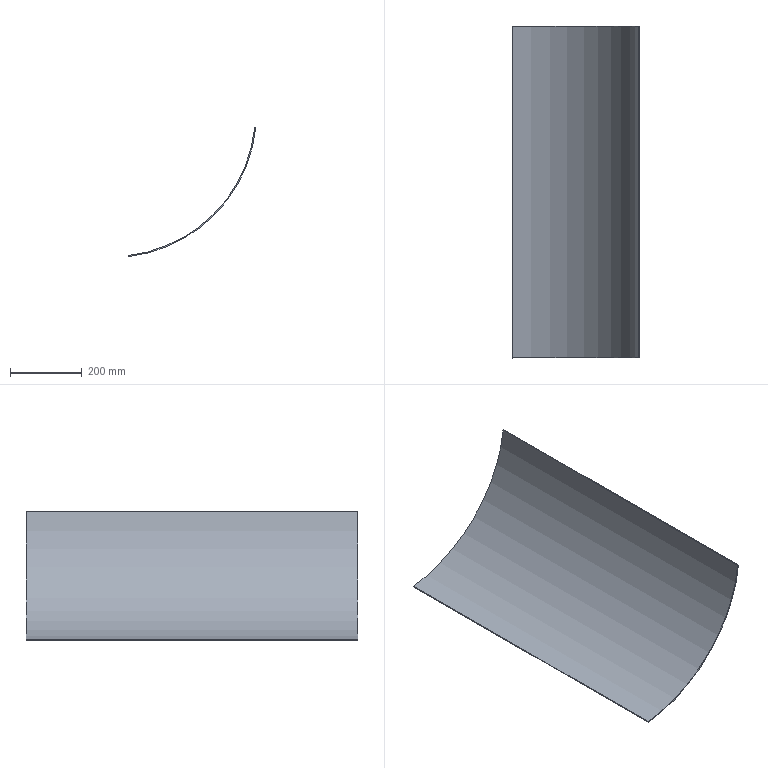Part | NX | features DATUM_CSYS 2, EXTRUDE 1, SKETCH 1 | 1 solid | 6 faces | box 355.98 x 926 x 360.442 mm | volume 1514546 mm3 | plane 4 | cylinder 2 | commonest cylinder face diameters 800 x1 806 x1
STEP:
#1=CARTESIAN_POINT('',(45.,463.,-397.461));
#2=VERTEX_POINT('',#1);
#3=CARTESIAN_POINT('',(45.337,463.,-400.442));
#4=VERTEX_POINT('',#3);
#5=CARTESIAN_POINT('',(45.,463.,-397.461));
#6=DIRECTION('',(0.1125,0.,-0.9937));
#7=VECTOR('',#6,1000.);
#8=LINE('',#5,#7);
#9=EDGE_CURVE('',#2,#4,#8,.T.);
#10=ORIENTED_EDGE('',*,*,#9,.F.);
#11=CARTESIAN_POINT('',(397.995,463.,-40.));
#12=VERTEX_POINT('',#11);
#13=CARTESIAN_POINT('',(0.,463.,0.));
#14=DIRECTION('',(0.,-1.,0.));
#15=DIRECTION('',(1.,0.,0.));
#16=AXIS2_PLACEMENT_3D('',#13,#14,#15);
#17=CIRCLE('',#16,400.);
#18=EDGE_CURVE('',#2,#12,#17,.T.);
#19=ORIENTED_EDGE('',*,*,#18,.T.);
#20=CARTESIAN_POINT('',(400.98,463.,-40.3));
#21=VERTEX_POINT('',#20);
#22=CARTESIAN_POINT('',(397.995,463.,-40.));
#23=DIRECTION('',(0.995,0.,-0.1));
#24=VECTOR('',#23,1000.);
#25=LINE('',#22,#24);
#26=EDGE_CURVE('',#12,#21,#25,.T.);
#27=ORIENTED_EDGE('',*,*,#26,.T.);
#28=CARTESIAN_POINT('',(0.,463.,0.));
#29=DIRECTION('',(0.,-1.,0.));
#30=DIRECTION('',(0.,0.,-1.));
#31=AXIS2_PLACEMENT_3D('',#28,#29,#30);
#32=CIRCLE('',#31,403.);
#33=EDGE_CURVE('',#4,#21,#32,.T.);
#34=ORIENTED_EDGE('',*,*,#33,.F.);
#35=EDGE_LOOP('',(#10,#19,#27,#34));
#36=FACE_BOUND('',#35,.T.);
#37=CARTESIAN_POINT('',(0.,463.,0.));
#38=DIRECTION('',(0.,1.,0.));
#39=DIRECTION('',(0.,0.,1.));
#40=AXIS2_PLACEMENT_3D('',#37,#38,#39);
#41=PLANE('',#40);
#42=ADVANCED_FACE('',(#36),#41,.T.);
#43=ORIENTED_EDGE('',*,*,#26,.F.);
#44=CARTESIAN_POINT('',(397.995,-463.,-40.));
#45=VERTEX_POINT('',#44);
#46=CARTESIAN_POINT('',(397.995,463.,-40.));
#47=DIRECTION('',(0.,-1.,0.));
#48=VECTOR('',#47,1000.);
#49=LINE('',#46,#48);
#50=EDGE_CURVE('',#12,#45,#49,.T.);
#51=ORIENTED_EDGE('',*,*,#50,.T.);
#52=CARTESIAN_POINT('',(400.98,-463.,-40.3));
#53=VERTEX_POINT('',#52);
#54=CARTESIAN_POINT('',(397.995,-463.,-40.));
#55=DIRECTION('',(0.995,0.,-0.1));
#56=VECTOR('',#55,1000.);
#57=LINE('',#54,#56);
#58=EDGE_CURVE('',#45,#53,#57,.T.);
#59=ORIENTED_EDGE('',*,*,#58,.T.);
#60=CARTESIAN_POINT('',(400.98,463.,-40.3));
#61=DIRECTION('',(0.,-1.,0.));
#62=VECTOR('',#61,1000.);
#63=LINE('',#60,#62);
#64=EDGE_CURVE('',#21,#53,#63,.T.);
#65=ORIENTED_EDGE('',*,*,#64,.F.);
#66=EDGE_LOOP('',(#43,#51,#59,#65));
#67=FACE_BOUND('',#66,.T.);
#68=CARTESIAN_POINT('',(397.995,0.,-40.));
#69=DIRECTION('',(0.1,0.,0.995));
#70=DIRECTION('',(0.,-1.,0.));
#71=AXIS2_PLACEMENT_3D('',#68,#69,#70);
#72=PLANE('',#71);
#73=ADVANCED_FACE('',(#67),#72,.T.);
#74=ORIENTED_EDGE('',*,*,#58,.F.);
#75=CARTESIAN_POINT('',(45.,-463.,-397.461));
#76=VERTEX_POINT('',#75);
#77=CARTESIAN_POINT('',(0.,-463.,0.));
#78=DIRECTION('',(0.,-1.,0.));
#79=DIRECTION('',(1.,0.,0.));
#80=AXIS2_PLACEMENT_3D('',#77,#78,#79);
#81=CIRCLE('',#80,400.);
#82=EDGE_CURVE('',#76,#45,#81,.T.);
#83=ORIENTED_EDGE('',*,*,#82,.F.);
#84=CARTESIAN_POINT('',(45.337,-463.,-400.442));
#85=VERTEX_POINT('',#84);
#86=CARTESIAN_POINT('',(45.,-463.,-397.461));
#87=DIRECTION('',(0.1125,0.,-0.9937));
#88=VECTOR('',#87,1000.);
#89=LINE('',#86,#88);
#90=EDGE_CURVE('',#76,#85,#89,.T.);
#91=ORIENTED_EDGE('',*,*,#90,.T.);
#92=CARTESIAN_POINT('',(0.,-463.,0.));
#93=DIRECTION('',(0.,-1.,0.));
#94=DIRECTION('',(0.,0.,-1.));
#95=AXIS2_PLACEMENT_3D('',#92,#93,#94);
#96=CIRCLE('',#95,403.);
#97=EDGE_CURVE('',#85,#53,#96,.T.);
#98=ORIENTED_EDGE('',*,*,#97,.T.);
#99=EDGE_LOOP('',(#74,#83,#91,#98));
#100=FACE_BOUND('',#99,.T.);
#101=CARTESIAN_POINT('',(0.,-463.,0.));
#102=DIRECTION('',(0.,1.,0.));
#103=DIRECTION('',(0.,0.,1.));
#104=AXIS2_PLACEMENT_3D('',#101,#102,#103);
#105=PLANE('',#104);
#106=ADVANCED_FACE('',(#100),#105,.F.);
#107=CARTESIAN_POINT('',(45.,463.,-397.461));
#108=DIRECTION('',(0.,-1.,0.));
#109=VECTOR('',#108,1000.);
#110=LINE('',#107,#109);
#111=EDGE_CURVE('',#2,#76,#110,.T.);
#112=ORIENTED_EDGE('',*,*,#111,.F.);
#113=ORIENTED_EDGE('',*,*,#9,.T.);
#114=CARTESIAN_POINT('',(45.337,463.,-400.442));
#115=DIRECTION('',(0.,-1.,0.));
#116=VECTOR('',#115,1000.);
#117=LINE('',#114,#116);
#118=EDGE_CURVE('',#4,#85,#117,.T.);
#119=ORIENTED_EDGE('',*,*,#118,.T.);
#120=ORIENTED_EDGE('',*,*,#90,.F.);
#121=EDGE_LOOP('',(#112,#113,#119,#120));
#122=FACE_BOUND('',#121,.T.);
#123=CARTESIAN_POINT('',(45.,0.,-397.461));
#124=DIRECTION('',(0.9937,0.,0.1125));
#125=DIRECTION('',(0.,-1.,0.));
#126=AXIS2_PLACEMENT_3D('',#123,#124,#125);
#127=PLANE('',#126);
#128=ADVANCED_FACE('',(#122),#127,.F.);
#129=ORIENTED_EDGE('',*,*,#97,.F.);
#130=ORIENTED_EDGE('',*,*,#118,.F.);
#131=ORIENTED_EDGE('',*,*,#33,.T.);
#132=ORIENTED_EDGE('',*,*,#64,.T.);
#133=EDGE_LOOP('',(#129,#130,#131,#132));
#134=FACE_BOUND('',#133,.T.);
#135=CARTESIAN_POINT('',(0.,463.,0.));
#136=DIRECTION('',(0.,-1.,0.));
#137=DIRECTION('',(0.,0.,-1.));
#138=AXIS2_PLACEMENT_3D('',#135,#136,#137);
#139=CYLINDRICAL_SURFACE('',#138,403.);
#140=ADVANCED_FACE('',(#134),#139,.T.);
#141=ORIENTED_EDGE('',*,*,#82,.T.);
#142=ORIENTED_EDGE('',*,*,#50,.F.);
#143=ORIENTED_EDGE('',*,*,#18,.F.);
#144=ORIENTED_EDGE('',*,*,#111,.T.);
#145=EDGE_LOOP('',(#141,#142,#143,#144));
#146=FACE_BOUND('',#145,.T.);
#147=CARTESIAN_POINT('',(0.,463.,0.));
#148=DIRECTION('',(0.,-1.,0.));
#149=DIRECTION('',(0.,0.,-1.));
#150=AXIS2_PLACEMENT_3D('',#147,#148,#149);
#151=CYLINDRICAL_SURFACE('',#150,400.);
#152=ADVANCED_FACE('',(#146),#151,.F.);
#153=CLOSED_SHELL('',(#42,#73,#106,#128,#140,#152));
#154=MANIFOLD_SOLID_BREP('',#153);
#155=(LENGTH_UNIT()NAMED_UNIT(*)SI_UNIT(.MILLI.,.METRE.));
#156=UNCERTAINTY_MEASURE_WITH_UNIT(LENGTH_MEASURE(0.00001),#155,'','');
#157=(NAMED_UNIT(*)PLANE_ANGLE_UNIT()SI_UNIT($,.RADIAN.));
#158=(NAMED_UNIT(*)SI_UNIT($,.STERADIAN.)SOLID_ANGLE_UNIT());
#159=(GEOMETRIC_REPRESENTATION_CONTEXT(3)GLOBAL_UNCERTAINTY_ASSIGNED_CONTEXT((#156))GLOBAL_UNIT_ASSIGNED_CONTEXT((#155,#157,#158))REPRESENTATION_CONTEXT('',''));
#160=ADVANCED_BREP_SHAPE_REPRESENTATION('',(#154),#159);